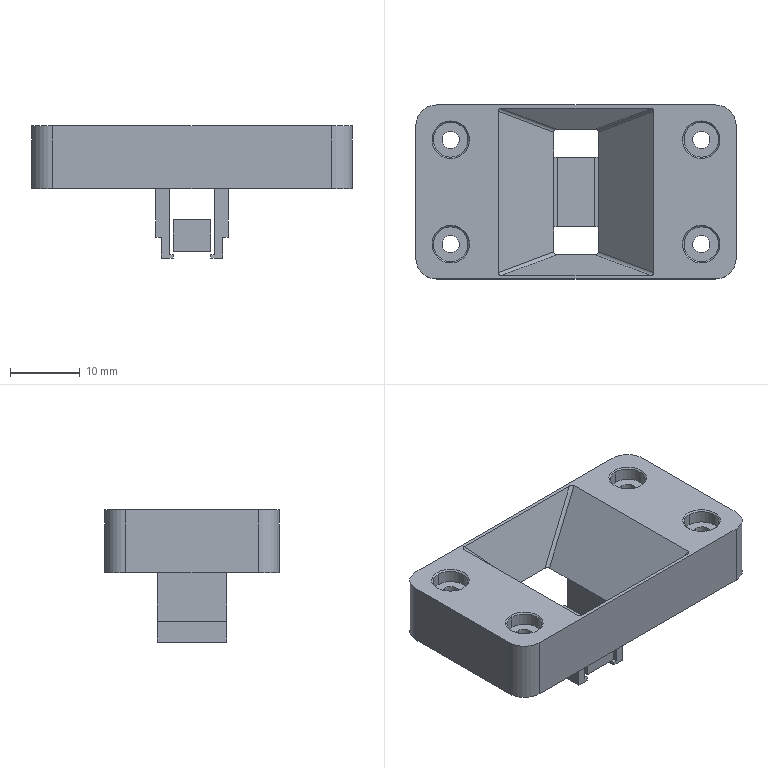NC program | NX | posted with a generic post | part box 46 x 25 x 19 mm
Lines 1575 to 3677 of 3737, first 1767 of 2099 lines:
(FIXED_CONTOUR_COPY , TOOL : D2R0.2)
N3094 T05 M6
N3096 G54
N3098 G17 G0 G90 X-10.255 Y11.119 S9500 M3
N3100 G43 Z30. H5
N3102 Z3.2
N3104 G94 G1 Z1.672 F500.
N3106 X-10.383 Y10.99 Z0.082
N3108 X-10.316 Y11.058 Z0.006 F2500.
N3110 X-10.3 Y11.073 Z0.052
N3112 X-10.229
N3114 X-10.264 Y11.039 Z-0.052
N3116 X-10.383 Y10.919 Z0.082
N3118 Y10.848
N3120 X-10.212 Y11.019 Z-0.11
N3122 X-10.158 Y11.073 Z0.052
N3124 X-10.087
N3126 X-10.161 Y11. Z-0.168
N3128 X-10.383 Y10.777 Z0.082
N3130 Y10.706
N3132 X-10.109 Y10.98 Z-0.226
N3134 X-10.016 Y11.073 Z0.053
N3136 X-9.945 Y11.074
N3138 X-10.058 Y10.961 Z-0.284
N3140 X-10.383 Y10.635 Z0.082
N3142 Y10.564
N3144 X-10.006 Y10.942 Z-0.342
N3146 X-9.874 Y11.074 Z0.053
N3148 X-9.803
N3150 X-9.954 Y10.922 Z-0.4
N3152 X-10.383 Y10.494 Z0.082
N3154 Y10.423
N3156 X-9.903 Y10.903 Z-0.458
N3158 X-9.732 Y11.074 Z0.053
N3160 X-9.662
N3162 X-9.851 Y10.884 Z-0.516
N3164 X-10.383 Y10.352 Z0.082
N3166 Y10.281
N3168 X-9.8 Y10.864 Z-0.574
N3170 X-9.591 Y11.074 Z0.053
N3172 X-9.52
N3174 X-9.748 Y10.845 Z-0.632
N3176 X-10.383 Y10.21 Z0.082
N3178 Y10.139
N3180 X-9.697 Y10.826 Z-0.69
N3182 X-9.449 Y11.074 Z0.053
N3184 X-9.378
N3186 X-9.645 Y10.806 Z-0.748
N3188 X-10.383 Y10.068 Z0.082
N3190 Y9.997
N3192 X-9.593 Y10.787 Z-0.806
N3194 X-9.307 Y11.074 Z0.053
N3196 X-9.236
N3198 X-9.542 Y10.768 Z-0.864
N3200 X-10.383 Y9.926 Z0.082
N3202 Y9.855
N3204 X-9.49 Y10.748 Z-0.922
N3206 X-9.165 Y11.074 Z0.053
N3208 X-9.094
N3210 X-9.439 Y10.729 Z-0.98
N3212 X-10.383 Y9.784 Z0.082
N3214 Y9.714
N3216 X-9.387 Y10.71 Z-1.038
N3218 X-9.023 Y11.074 Z0.053
N3220 X-8.952
N3222 X-9.336 Y10.69 Z-1.096
N3224 X-10.383 Y9.643 Z0.082
N3226 Y9.572
N3228 X-9.284 Y10.671 Z-1.154
N3230 X-8.881 Y11.074 Z0.053
N3232 X-8.811
N3234 X-9.232 Y10.652 Z-1.212
N3236 X-10.383 Y9.501 Z0.082
N3238 Y9.43
N3240 X-9.181 Y10.632 Z-1.27
N3242 X-8.74 Y11.074 Z0.053
N3244 X-8.669
N3246 X-9.129 Y10.613 Z-1.328
N3248 X-10.383 Y9.359 Z0.082
N3250 Y9.288
N3252 X-9.078 Y10.594 Z-1.387
N3254 X-8.598 Y11.074 Z0.053
N3256 X-8.527
N3258 X-9.026 Y10.574 Z-1.445
N3260 X-10.383 Y9.217 Z0.082
N3262 Y9.146
N3264 X-8.975 Y10.555 Z-1.503
N3266 X-8.456 Y11.074 Z0.053
N3268 X-8.385
N3270 X-8.923 Y10.536 Z-1.561
N3272 X-10.383 Y9.075 Z0.082
N3274 Y9.004
N3276 X-8.871 Y10.516 Z-1.619
N3278 X-8.314 Y11.074 Z0.053
N3280 X-8.243
N3282 X-8.82 Y10.497 Z-1.677
N3284 X-10.383 Y8.933 Z0.082
N3286 Y8.863
N3288 X-8.768 Y10.478 Z-1.735
N3290 X-8.172 Y11.074 Z0.053
N3292 X-8.101
N3294 X-8.717 Y10.458 Z-1.793
N3296 X-10.383 Y8.792 Z0.082
N3298 Y8.721
N3300 X-8.665 Y10.439 Z-1.851
N3302 X-8.031 Y11.074 Z0.053
N3304 X-7.96
N3306 X-8.614 Y10.42 Z-1.909
N3308 X-10.383 Y8.65 Z0.082
N3310 Y8.579
N3312 X-8.562 Y10.4 Z-1.967
N3314 X-7.889 Y11.074 Z0.053
N3316 X-7.818
N3318 X-8.51 Y10.381 Z-2.025
N3320 X-10.383 Y8.508 Z0.082
N3322 Y8.437
N3324 X-8.459 Y10.362 Z-2.083
N3326 X-7.747 Y11.074 Z0.053
N3328 X-7.676
N3330 X-8.407 Y10.342 Z-2.141
N3332 X-10.383 Y8.366 Z0.082
N3334 Y8.295
N3336 X-8.356 Y10.323 Z-2.199
N3338 X-7.605 Y11.074 Z0.053
N3340 X-7.534
N3342 X-8.304 Y10.304 Z-2.257
N3344 X-10.383 Y8.224 Z0.082
N3346 Y8.153
N3348 X-8.253 Y10.284 Z-2.315
N3350 X-7.463 Y11.074 Z0.053
N3352 X-7.392
N3354 X-8.201 Y10.265 Z-2.373
N3356 X-10.383 Y8.083 Z0.082
N3358 Y8.012
N3360 X-8.149 Y10.246 Z-2.431
N3362 X-7.321 Y11.074 Z0.053
N3364 X-7.251
N3366 X-8.098 Y10.226 Z-2.489
N3368 X-10.383 Y7.941 Z0.082
N3370 Y7.87
N3372 X-8.046 Y10.207 Z-2.547
N3374 X-7.18 Y11.074 Z0.053
N3376 X-7.109
N3378 X-7.995 Y10.188 Z-2.605
N3380 X-10.383 Y7.799 Z0.082
N3382 Y7.728
N3384 X-7.943 Y10.168 Z-2.663
N3386 X-7.038 Y11.074 Z0.053
N3388 X-6.967
N3390 X-7.892 Y10.149 Z-2.721
N3392 X-10.383 Y7.657 Z0.082
N3394 Y7.586
N3396 X-7.84 Y10.13 Z-2.779
N3398 X-6.896 Y11.074 Z0.053
N3400 X-6.825
N3402 X-7.788 Y10.11 Z-2.837
N3404 X-10.383 Y7.515 Z0.082
N3406 Y7.444
N3408 X-7.737 Y10.091 Z-2.895
N3410 X-6.754 Y11.074 Z0.053
N3412 X-6.683
N3414 X-7.685 Y10.072 Z-2.953
N3416 X-10.383 Y7.373 Z0.082
N3418 Y7.302
N3420 X-7.634 Y10.052 Z-3.011
N3422 X-6.612 Y11.074 Z0.053
N3424 X-6.541
N3426 X-7.582 Y10.033 Z-3.069
N3428 X-10.383 Y7.232 Z0.082
N3430 Y7.161
N3432 X-7.531 Y10.013 Z-3.127
N3434 X-6.47 Y11.074 Z0.053
N3436 X-6.4
N3438 X-7.479 Y9.994 Z-3.185
N3440 X-10.383 Y7.09 Z0.082
N3442 Y7.019
N3444 X-7.427 Y9.975 Z-3.243
N3446 X-6.329 Y11.074 Z0.053
N3448 X-6.258
N3450 X-7.376 Y9.955 Z-3.301
N3452 X-10.383 Y6.948 Z0.082
N3454 Y6.877
N3456 X-7.324 Y9.936 Z-3.359
N3458 X-6.187 Y11.074 Z0.053
N3460 X-6.116
N3462 X-7.273 Y9.917 Z-3.417
N3464 X-10.383 Y6.806 Z0.082
N3466 Y6.735
N3468 X-7.221 Y9.897 Z-3.475
N3470 X-6.045 Y11.074 Z0.053
N3472 X-5.974
N3474 X-7.17 Y9.878 Z-3.533
N3476 X-10.383 Y6.664 Z0.082
N3478 Y6.593
N3480 X-7.118 Y9.859 Z-3.591
N3482 X-5.903 Y11.074 Z0.053
N3484 X-5.832
N3486 X-7.066 Y9.839 Z-3.649
N3488 X-10.383 Y6.522 Z0.082
N3490 Y6.452
N3492 X-7.015 Y9.82 Z-3.707
N3494 X-5.761 Y11.074 Z0.053
N3496 X-5.69
N3498 X-6.963 Y9.801 Z-3.765
N3500 X-10.383 Y6.381 Z0.082
N3502 Y6.31
N3504 X-6.912 Y9.781 Z-3.823
N3506 X-5.62 Y11.074 Z0.053
N3508 X-5.549
N3510 X-6.86 Y9.762 Z-3.881
N3512 X-10.383 Y6.239 Z0.082
N3514 Y6.168
N3516 X-6.809 Y9.743 Z-3.939
N3518 X-5.478 Y11.074 Z0.053
N3520 X-5.407
N3522 X-6.757 Y9.723 Z-3.997
N3524 X-10.383 Y6.097 Z0.082
N3526 Y6.026
N3528 X-6.705 Y9.704 Z-4.055
N3530 X-5.336 Y11.074 Z0.053
N3532 X-5.265
N3534 X-6.654 Y9.685 Z-4.113
N3536 X-10.383 Y5.955 Z0.082
N3538 Y5.884
N3540 X-6.602 Y9.665 Z-4.171
N3542 X-5.194 Y11.074 Z0.053
N3544 X-5.123
N3546 X-6.551 Y9.646 Z-4.229
N3548 X-10.383 Y5.813 Z0.082
N3550 Y5.742
N3552 X-6.499 Y9.627 Z-4.287
N3554 X-5.052 Y11.074 Z0.053
N3556 X-4.981
N3558 X-6.448 Y9.607 Z-4.345
N3560 X-10.383 Y5.671 Z0.082
N3562 Y5.601
N3564 X-6.396 Y9.588 Z-4.404
N3566 X-4.91 Y11.074 Z0.053
N3568 X-4.839
N3570 X-6.344 Y9.569 Z-4.462
N3572 X-10.383 Y5.53 Z0.082
N3574 Y5.459
N3576 X-6.293 Y9.549 Z-4.52
N3578 X-4.769 Y11.074 Z0.053
N3580 X-4.698
N3582 X-6.241 Y9.53 Z-4.578
N3584 X-10.383 Y5.388 Z0.082
N3586 Y5.317
N3588 X-6.19 Y9.511 Z-4.636
N3590 X-4.627 Y11.074 Z0.053
N3592 X-4.556
N3594 X-6.138 Y9.491 Z-4.694
N3596 X-10.383 Y5.246 Z0.082
N3598 Y5.175
N3600 X-6.087 Y9.472 Z-4.752
N3602 X-4.485 Y11.074 Z0.053
N3604 X-4.414
N3606 X-6.035 Y9.453 Z-4.81
N3608 X-10.383 Y5.104 Z0.082
N3610 Y5.033
N3612 X-5.983 Y9.433 Z-4.868
N3614 X-4.343 Y11.074 Z0.053
N3616 X-4.272
N3618 X-5.932 Y9.414 Z-4.926
N3620 X-10.383 Y4.962 Z0.082
N3622 Y4.891
N3624 X-5.88 Y9.395 Z-4.984
N3626 X-4.201 Y11.074 Z0.053
N3628 X-4.13
N3630 X-5.829 Y9.375 Z-5.042
N3632 X-10.383 Y4.821 Z0.082
N3634 Y4.75
N3636 X-5.777 Y9.356 Z-5.1
N3638 X-4.059 Y11.074 Z0.053
N3640 X-3.989
N3642 X-5.726 Y9.337 Z-5.158
N3644 X-10.383 Y4.679 Z0.082
N3646 Y4.608
N3648 X-5.674 Y9.317 Z-5.216
N3650 X-3.918 Y11.074 Z0.053
N3652 X-3.847
N3654 X-5.622 Y9.298 Z-5.274
N3656 X-10.383 Y4.537 Z0.082
N3658 Y4.466
N3660 X-5.571 Y9.279 Z-5.332
N3662 X-3.776 Y11.074 Z0.053
N3664 X-3.705
N3666 X-5.519 Y9.259 Z-5.39
N3668 X-10.383 Y4.395 Z0.082
N3670 Y4.324
N3672 X-5.468 Y9.24 Z-5.448
N3674 X-3.634 Y11.074 Z0.053
N3676 X-3.563
N3678 X-5.416 Y9.221 Z-5.506
N3680 X-10.383 Y4.253 Z0.082
N3682 Y4.182
N3684 X-5.365 Y9.201 Z-5.564
N3686 X-3.492 Y11.074 Z0.053
N3688 X-3.421
N3690 X-5.313 Y9.182 Z-5.622
N3692 X-10.383 Y4.111 Z0.082
N3694 Y4.04
N3696 X-5.261 Y9.163 Z-5.68
N3698 X-3.35 Y11.074 Z0.053
N3700 X-3.279
N3702 X-5.21 Y9.143 Z-5.738
N3704 X-10.383 Y3.97 Z0.082
N3706 Y3.899
N3708 X-5.158 Y9.124 Z-5.796
N3710 X-3.209 Y11.074 Z0.053
N3712 X-3.138
N3714 X-5.107 Y9.105 Z-5.854
N3716 X-10.383 Y3.828 Z0.082
N3718 Y3.757
N3720 X-5.055 Y9.085 Z-5.912
N3722 X-3.067 Y11.074 Z0.053
N3724 X-2.996
N3726 X-5.003 Y9.066 Z-5.97
N3728 X-10.383 Y3.686 Z0.082
N3730 Y3.615
N3732 X-4.952 Y9.046 Z-6.028
N3734 X-2.925 Y11.074 Z0.053
N3736 X-2.854
N3738 X-4.9 Y9.027 Z-6.086
N3740 X-10.383 Y3.544 Z0.082
N3742 Y3.473
N3744 X-4.849 Y9.008 Z-6.144
N3746 X-2.783 Y11.074 Z0.053
N3748 X-2.712
N3750 X-4.797 Y8.988 Z-6.202
N3752 X-10.383 Y3.402 Z0.082
N3754 Y3.331
N3756 X-4.746 Y8.969 Z-6.26
N3758 X-2.641 Y11.074 Z0.053
N3760 X-2.57
N3762 X-4.694 Y8.95 Z-6.318
N3764 X-10.383 Y3.26 Z0.082
N3766 Y3.19
N3768 X-4.642 Y8.93 Z-6.376
N3770 X-2.499 Y11.074 Z0.053
N3772 X-2.428
N3774 X-4.591 Y8.911 Z-6.434
N3776 X-10.383 Y3.119 Z0.082
N3778 Y3.048
N3780 X-4.539 Y8.892 Z-6.492
N3782 X-2.358 Y11.074 Z0.053
N3784 X-2.287
N3786 X-4.488 Y8.872 Z-6.55
N3788 X-10.383 Y2.977 Z0.082
N3790 Y2.906
N3792 X-4.436 Y8.853 Z-6.608
N3794 X-2.216 Y11.074 Z0.053
N3796 X-2.145
N3798 X-4.385 Y8.834 Z-6.666
N3800 X-10.383 Y2.835 Z0.082
N3802 Y2.764
N3804 X-4.333 Y8.814 Z-6.724
N3806 X-2.074 Y11.074 Z0.053
N3808 X-2.003
N3810 X-4.281 Y8.795 Z-6.782
N3812 X-10.383 Y2.693 Z0.082
N3814 Y2.622
N3816 X-4.23 Y8.776 Z-6.84
N3818 X-1.932 Y11.074 Z0.053
N3820 X-1.861
N3822 X-4.178 Y8.756 Z-6.898
N3824 X-10.383 Y2.551 Z0.082
N3826 Y2.48
N3828 X-4.127 Y8.737 Z-6.956
N3830 X-1.79 Y11.074 Z0.053
N3832 X-1.719
N3834 X-4.075 Y8.718 Z-7.014
N3836 X-10.383 Y2.409 Z0.082
N3838 Y2.339
N3840 X-4.024 Y8.698 Z-7.072
N3842 X-1.648 Y11.074 Z0.053
N3844 X-1.578
N3846 X-3.972 Y8.679 Z-7.13
N3848 X-10.383 Y2.268 Z0.082
N3850 Y2.197
N3852 X-3.92 Y8.66 Z-7.188
N3854 X-1.507 Y11.074 Z0.053
N3856 X-1.436
N3858 X-3.869 Y8.64 Z-7.246
N3860 X-10.383 Y2.126 Z0.082
N3862 Y2.055
N3864 X-3.817 Y8.621 Z-7.304
N3866 X-1.365 Y11.074 Z0.053
N3868 X-1.294
N3870 X-3.766 Y8.602 Z-7.362
N3872 X-10.383 Y1.984 Z0.082
N3874 Y1.913
N3876 X-3.714 Y8.582 Z-7.421
N3878 X-1.223 Y11.074 Z0.053
N3880 X-1.152
N3882 X-3.663 Y8.563 Z-7.479
N3884 X-10.383 Y1.842 Z0.082
N3886 Y1.771
N3888 X-3.611 Y8.544 Z-7.537
N3890 X-1.081 Y11.074 Z0.053
N3892 X-1.01
N3894 X-3.559 Y8.524 Z-7.595
N3896 X-10.383 Y1.7 Z0.082
N3898 Y1.629
N3900 X-3.508 Y8.505 Z-7.653
N3902 X-0.939 Y11.074 Z0.053
N3904 X-0.868
N3906 X-3.456 Y8.486 Z-7.711
N3908 X-10.383 Y1.559 Z0.082
N3910 Y1.488
N3912 X-3.405 Y8.466 Z-7.769
N3914 X-0.797 Y11.074 Z0.053
N3916 X-0.727
N3918 X-3.353 Y8.447 Z-7.827
N3920 X-10.383 Y1.417 Z0.082
N3922 Y1.346
N3924 X-3.302 Y8.428 Z-7.885
N3926 X-0.656 Y11.074 Z0.053
N3928 X-0.585
N3930 X-3.25 Y8.408 Z-7.943
N3932 X-10.383 Y1.275 Z0.082
N3934 Y1.204
N3936 X-3.198 Y8.389 Z-8.001
N3938 X-0.514 Y11.074 Z0.053
N3940 X-0.443
N3942 X-3.147 Y8.37 Z-8.059
N3944 X-10.383 Y1.133 Z0.082
N3946 Y1.062
N3948 X-3.095 Y8.35 Z-8.117
N3950 X-0.372 Y11.074 Z0.053
N3952 X-0.301
N3954 X-3.044 Y8.331 Z-8.175
N3956 X-10.383 Y0.991 Z0.082
N3958 Y0.92
N3960 X-2.992 Y8.312 Z-8.233
N3962 X-0.23 Y11.074 Z0.053
N3964 X-0.159
N3966 X-2.941 Y8.292 Z-8.291
N3968 X-10.383 Y0.849 Z0.082
N3970 Y0.779
N3972 X-2.889 Y8.273 Z-8.349
N3974 X-0.088 Y11.074 Z0.053
N3976 X-0.017
N3978 X-2.837 Y8.254 Z-8.407
N3980 X-10.383 Y0.708 Z0.082
N3982 Y0.637
N3984 X-2.786 Y8.234 Z-8.465
N3986 X0.053 Y11.074 Z0.053
N3988 X0.124
N3990 X-2.734 Y8.215 Z-8.523
N3992 X-10.383 Y0.566 Z0.082
N3994 Y0.495
N3996 X-2.683 Y8.196 Z-8.581
N3998 X0.195 Y11.074 Z0.053
N4000 X0.266
N4002 X-2.631 Y8.176 Z-8.639
N4004 X-10.383 Y0.424 Z0.082
N4006 Y0.353
N4008 X-2.58 Y8.157 Z-8.697
N4010 X0.337 Y11.074 Z0.053
N4012 X0.408
N4014 X-2.528 Y8.138 Z-8.755
N4016 X-10.383 Y0.282 Z0.082
N4018 Y0.211
N4020 X-2.476 Y8.118 Z-8.813
N4022 X0.479 Y11.074 Z0.053
N4024 X0.55
N4026 X-2.425 Y8.099 Z-8.871
N4028 X-10.383 Y0.14 Z0.082
N4030 Y0.069
N4032 X-2.373 Y8.08 Z-8.929
N4034 X0.621 Y11.074 Z0.053
N4036 X0.692
N4038 X-2.322 Y8.06 Z-8.987
N4040 X-10.383 Y-0.002 Z0.082
N4042 Y-0.072
N4044 X-2.27 Y8.041 Z-9.045
N4046 X0.763 Y11.074 Z0.053
N4048 X0.834
N4050 X-2.219 Y8.021 Z-9.103
N4052 X-10.383 Y-0.143 Z0.082
N4054 Y-0.214
N4056 X-2.167 Y8.002 Z-9.161
N4058 X0.904 Y11.074 Z0.053
N4060 X0.988
N4062 X-2.106 Y7.979 Z-9.231
N4064 X-2.1 Y7.976 Z-9.239
N4066 X-2.085 Y7.967 Z-9.266
N4068 X-2.084 Y7.966 Z-9.269
N4070 X-2.083 Z-9.271
N4072 X-2.077 Y7.96 Z-9.288
N4074 X-2.072 Y7.956 Z-9.3
N4076 X-2.068 Y7.947 Z-9.326
N4078 X-2.054
N4080 X1.072 Y11.074 Z0.053
N4082 X1.156
N4084 X-1.97 Y7.947 Z-9.326
N4086 X-1.887
N4088 X1.24 Y11.074 Z0.053
N4090 X1.324
N4092 X-1.803 Y7.947 Z-9.326
N4094 X-1.719
N4096 X1.408 Y11.074 Z0.053
N4098 X1.492
N4100 X-1.635 Y7.947 Z-9.326
N4102 X-1.551
N4104 X1.576 Y11.074 Z0.053
N4106 X1.66
N4108 X-1.467 Y7.947 Z-9.326
N4110 X-1.383
N4112 X1.743 Y11.074 Z0.053
N4114 X1.827
N4116 X-1.299 Y7.947 Z-9.326
N4118 X-1.215
N4120 X1.911 Y11.074 Z0.053
N4122 X1.995
N4124 X-1.132 Y7.947 Z-9.326
N4126 X-1.048
N4128 X2.079 Y11.074 Z0.053
N4130 X2.163
N4132 X-0.964 Y7.947 Z-9.326
N4134 X-0.88
N4136 X2.247 Y11.074 Z0.053
N4138 X2.331
N4140 X-0.796 Y7.947 Z-9.326
N4142 X-0.712
N4144 X2.415 Y11.074 Z0.053
N4146 X2.499
N4148 X-0.628 Y7.947 Z-9.326
N4150 X-0.544
N4152 X2.582 Y11.074 Z0.053
N4154 X2.666
N4156 X-0.46 Y7.947 Z-9.326
N4158 X-0.376
N4160 X2.75 Y11.074 Z0.053
N4162 X2.834
N4164 X-0.293 Y7.947 Z-9.326
N4166 X-0.209
N4168 X2.918 Y11.074 Z0.053
N4170 X3.002
N4172 X-0.125 Y7.947 Z-9.326
N4174 X-0.041
N4176 X3.086 Y11.074 Z0.053
N4178 X3.17
N4180 X0.043 Y7.947 Z-9.326
N4182 X0.127
N4184 X3.254 Y11.074 Z0.053
N4186 X3.337
N4188 X0.211 Y7.947 Z-9.326
N4190 X0.295
N4192 X3.421 Y11.074 Z0.053
N4194 X3.505
N4196 X0.379 Y7.947 Z-9.326
N4198 X0.463
N4200 X3.589 Y11.074 Z0.053
N4202 X3.673
N4204 X0.546 Y7.947 Z-9.326
N4206 X0.63
N4208 X3.757 Y11.074 Z0.053
N4210 X3.841
N4212 X0.714 Y7.947 Z-9.326
N4214 X0.798
N4216 X3.925 Y11.074 Z0.053
N4218 X4.009
N4220 X0.882 Y7.947 Z-9.326
N4222 X0.966
N4224 X4.093 Y11.074 Z0.053
N4226 X4.176
N4228 X1.05 Y7.947 Z-9.326
N4230 X1.134
N4232 X4.26 Y11.074 Z0.053
N4234 X4.344
N4236 X1.218 Y7.947 Z-9.326
N4238 X1.302
N4240 X4.428 Y11.074 Z0.053
N4242 X4.512
N4244 X1.385 Y7.947 Z-9.326
N4246 X1.469
N4248 X4.596 Y11.074 Z0.053
N4250 X4.68
N4252 X1.553 Y7.947 Z-9.326
N4254 X1.637
N4256 X4.764 Y11.074 Z0.053
N4258 X4.848
N4260 X1.721 Y7.947 Z-9.326
N4262 X1.805
N4264 X4.932 Y11.074 Z0.053
N4266 X5.015
N4268 X1.889 Y7.947 Z-9.326
N4270 X1.973
N4272 X5.099 Y11.074 Z0.053
N4274 X5.183
N4276 X2.057 Y7.947 Z-9.326
N4278 X2.068
N4280 X2.072 Y7.956 Z-9.3
N4282 X2.077 Y7.96 Z-9.288
N4284 X2.078 Y7.961 Z-9.285
N4286 X2.08 Y7.962 Z-9.281
N4288 X2.083 Y7.966 Z-9.271
N4290 X2.086 Y7.967 Z-9.266
N4292 X2.089 Y7.969 Z-9.259
N4294 X2.1 Y7.976 Z-9.239
N4296 X2.118 Y7.984 Z-9.215
N4298 Z-9.217
N4300 Y7.924
N4302 X2.213 Y8.019 Z-9.109
N4304 X5.267 Y11.074 Z0.053
N4306 X5.351
N4308 X2.347 Y8.07 Z-8.958
N4310 X2.118 Y7.84 Z-9.217
N4312 Y7.756
N4314 X2.482 Y8.12 Z-8.807
N4316 X5.435 Y11.074 Z0.053
N4318 X5.519
N4320 X2.616 Y8.17 Z-8.656
N4322 X2.118 Y7.672 Z-9.217
N4324 Y7.588
N4326 X2.75 Y8.221 Z-8.505
N4328 X5.603 Y11.074 Z0.053
N4330 X5.687
N4332 X2.884 Y8.271 Z-8.354
N4334 X2.118 Y7.504 Z-9.217
N4336 Y7.421
N4338 X3.018 Y8.321 Z-8.203
N4340 X5.771 Y11.074 Z0.053
N4342 X5.854
N4344 X3.153 Y8.372 Z-8.052
N4346 X2.118 Y7.337 Z-9.217
N4348 Y7.253
N4350 X3.287 Y8.422 Z-7.901
N4352 X5.938 Y11.074 Z0.053
N4354 X6.022
N4356 X3.421 Y8.472 Z-7.75
N4358 X2.118 Y7.169 Z-9.217
N4360 Y7.096
N4362 Y5.966 Z-8.085
N4364 Z-4.635
N4366 G0 Z-1.835
N4368 X1.924 Y7.033
N4370 Z-2.235
N4372 G1 Z-9.217 F500.
N4374 G3 X2.118 Y7.085 R0.2
N4376 G1 X3.555 Y8.523 Z-7.599 F2500.
N4378 X6.106 Y11.074 Z0.053
N4380 X6.19
N4382 X3.69 Y8.573 Z-7.448
N4384 X2.118 Y7.001 Z-9.217
N4386 Y6.917
N4388 X3.824 Y8.624 Z-7.297
N4390 X6.274 Y11.074 Z0.053
N4392 X6.358
N4394 X3.958 Y8.674 Z-7.146
N4396 X2.118 Y6.833 Z-9.217
N4398 Y6.749
N4400 X4.092 Y8.724 Z-6.995
N4402 X6.442 Y11.074 Z0.053
N4404 X6.526
N4406 X4.227 Y8.775 Z-6.844
N4408 X2.118 Y6.665 Z-9.217
N4410 Y6.582
N4412 X4.361 Y8.825 Z-6.693
N4414 X6.61 Y11.074 Z0.053
N4416 X6.694
N4418 X4.495 Y8.875 Z-6.542
N4420 X2.118 Y6.498 Z-9.217
N4422 Y6.414
N4424 X4.629 Y8.926 Z-6.391
N4426 X6.777 Y11.074 Z0.053
N4428 X6.861
N4430 X4.764 Y8.976 Z-6.24
N4432 X2.118 Y6.33 Z-9.217
N4434 Y6.246
N4436 X4.898 Y9.026 Z-6.089
N4438 X6.945 Y11.074 Z0.053
N4440 X7.029
N4442 X5.032 Y9.077 Z-5.938
N4444 X2.118 Y6.162 Z-9.217
N4446 Y6.078
N4448 X5.166 Y9.127 Z-5.787
N4450 X7.113 Y11.074 Z0.053
N4452 X7.197
N4454 X5.301 Y9.177 Z-5.636
N4456 X2.118 Y5.994 Z-9.217
N4458 Y5.91
N4460 X5.435 Y9.228 Z-5.485
N4462 X7.281 Y11.074 Z0.053
N4464 X7.365
N4466 X5.569 Y9.278 Z-5.334
N4468 X2.118 Y5.826 Z-9.217
N4470 Y5.742
N4472 X5.703 Y9.328 Z-5.183
N4474 X7.449 Y11.074 Z0.053
N4476 X7.533
N4478 X5.838 Y9.379 Z-5.032
N4480 X2.118 Y5.659 Z-9.217
N4482 Y5.575
N4484 X5.972 Y9.429 Z-4.881
N4486 X7.616 Y11.074 Z0.053
N4488 X7.7
N4490 X6.106 Y9.479 Z-4.73
N4492 X2.118 Y5.491 Z-9.217
N4494 Y5.407
N4496 X6.24 Y9.53 Z-4.579
N4498 X7.784 Y11.074 Z0.053
N4500 X7.868
N4502 X6.375 Y9.58 Z-4.428
N4504 X2.118 Y5.323 Z-9.217
N4506 Y5.239
N4508 X6.509 Y9.63 Z-4.276
N4510 X7.952 Y11.074 Z0.053
N4512 X8.036
N4514 X6.643 Y9.681 Z-4.126
N4516 X2.118 Y5.155 Z-9.217
N4518 Y5.071
N4520 X6.777 Y9.731 Z-3.974
N4522 X8.12 Y11.074 Z0.053
N4524 X8.204
N4526 X6.912 Y9.781 Z-3.823
N4528 X2.118 Y4.987 Z-9.217
N4530 Y4.903
N4532 X7.046 Y9.832 Z-3.672
N4534 X8.288 Y11.074 Z0.053
N4536 X8.372
N4538 X7.18 Y9.882 Z-3.521
N4540 X2.118 Y4.82 Z-9.217
N4542 Y4.736
N4544 X7.314 Y9.932 Z-3.37
N4546 X8.455 Y11.074 Z0.053
N4548 X8.539
N4550 X7.449 Y9.983 Z-3.219
N4552 X2.118 Y4.652 Z-9.217
N4554 Y4.568
N4556 X7.583 Y10.033 Z-3.068
N4558 X8.623 Y11.074 Z0.053
N4560 X8.707
N4562 X7.717 Y10.083 Z-2.917
N4564 X2.118 Y4.484 Z-9.217
N4566 Y4.4
N4568 X7.851 Y10.134 Z-2.766
N4570 X8.791 Y11.074 Z0.053
N4572 X8.875
N4574 X7.986 Y10.184 Z-2.615
N4576 X2.118 Y4.316 Z-9.217
N4578 Y4.232
N4580 X8.12 Y10.234 Z-2.464
N4582 X8.959 Y11.074 Z0.053
N4584 X9.043
N4586 X8.254 Y10.285 Z-2.313
N4588 X2.118 Y4.148 Z-9.217
N4590 Y4.064
N4592 X8.388 Y10.335 Z-2.162
N4594 X9.127 Y11.074 Z0.053
N4596 X9.211
N4598 X8.523 Y10.385 Z-2.011
N4600 X2.118 Y3.981 Z-9.217
N4602 Y3.897
N4604 X8.657 Y10.436 Z-1.86
N4606 X9.295 Y11.074 Z0.053
N4608 X9.378
N4610 X8.791 Y10.486 Z-1.709
N4612 X2.118 Y3.813 Z-9.217
N4614 Y3.729
N4616 X8.925 Y10.537 Z-1.558
N4618 X9.462 Y11.074 Z0.053
N4620 X9.546
N4622 X9.06 Y10.587 Z-1.407
N4624 X2.118 Y3.645 Z-9.217
N4626 Y3.561
N4628 X9.194 Y10.637 Z-1.256
N4630 X9.63 Y11.074 Z0.053
N4632 X9.714
N4634 X9.328 Y10.688 Z-1.105
N4636 X2.118 Y3.477 Z-9.217
N4638 Y3.393
N4640 X9.462 Y10.738 Z-0.954
N4642 X9.798 Y11.074 Z0.053
N4644 X9.882
N4646 X9.597 Y10.788 Z-0.803
N4648 X2.118 Y3.309 Z-9.217
N4650 Y3.225
N4652 X9.731 Y10.839 Z-0.652
N4654 X9.966 Y11.073 Z0.053
N4656 X10.05
N4658 X9.865 Y10.889 Z-0.501
N4660 X2.118 Y3.141 Z-9.217
N4662 Y3.058
N4664 X9.999 Y10.939 Z-0.35
N4666 X10.133 Y11.073 Z0.052
N4668 X10.217
N4670 X10.134 Y10.99 Z-0.199
N4672 X2.118 Y2.974 Z-9.217
N4674 Y2.89
N4676 X10.268 Y11.04 Z-0.048
N4678 X10.301 Y11.073 Z0.052
N4680 X10.356
N4682 X10.367 Y11.078 Z0.063
N4684 X10.383 Y11.086 Z0.082
N4686 Y11.06
N4688 X9.997 Y10.673 Z-0.353
N4690 X2.118 Y2.794 Z-9.217
N4692 Y2.699
N4694 X10.383 Y10.964 Z0.082
N4696 Y10.869
N4698 X2.118 Y2.603 Z-9.217
N4700 Y2.508
N4702 X10.383 Y10.773 Z0.082
N4704 Y10.678
N4706 X2.118 Y2.412 Z-9.217
N4708 Y2.317
N4710 X10.383 Y10.583 Z0.082
N4712 Y10.487
N4714 X2.118 Y2.221 Z-9.217
N4716 Y2.126
N4718 X10.383 Y10.392 Z0.082
N4720 Y10.296
N4722 X2.118 Y2.03 Z-9.217
N4724 Y1.935
N4726 X10.383 Y10.201 Z0.082
N4728 Y10.105
N4730 X2.118 Y1.839 Z-9.217
N4732 Y1.744
N4734 X10.383 Y10.01 Z0.082
N4736 Y9.914
N4738 X2.118 Y1.648 Z-9.217
N4740 Y1.553
N4742 X10.383 Y9.819 Z0.082
N4744 Y9.723
N4746 X2.118 Y1.457 Z-9.217
N4748 Y1.362
N4750 X10.383 Y9.628 Z0.082
N4752 Y9.544
N4754 X2.118 Y1.278 Z-9.217
N4756 Y1.194
N4758 X10.383 Y9.46 Z0.082
N4760 Y9.376
N4762 X2.118 Y1.11 Z-9.217
N4764 Y1.026
N4766 X10.383 Y9.292 Z0.082
N4768 Y9.208
N4770 X2.118 Y0.942 Z-9.217
N4772 Y0.858
N4774 X10.383 Y9.124 Z0.082
N4776 Y9.04
N4778 X2.118 Y0.774 Z-9.217
N4780 Y0.69
N4782 X10.383 Y8.956 Z0.082
N4784 Y8.872
N4786 X2.118 Y0.607 Z-9.217
N4788 Y0.523
N4790 X10.383 Y8.788 Z0.082
N4792 Y8.705
N4794 X2.118 Y0.439 Z-9.217
N4796 Y0.355
N4798 X10.383 Y8.621 Z0.082
N4800 Y8.537
N4802 X2.118 Y0.271 Z-9.217
N4804 Y0.187
N4806 X10.383 Y8.453 Z0.082
N4808 Y8.369
N4810 X2.118 Y0.103 Z-9.217
N4812 Y0.019
N4814 X10.383 Y8.285 Z0.082
N4816 Y8.201
N4818 X2.118 Y-0.065 Z-9.217
N4820 Y-0.149
N4822 X10.383 Y8.117 Z0.082
N4824 Y8.033
N4826 X2.118 Y-0.232 Z-9.217
N4828 Y-0.316
N4830 X10.383 Y7.949 Z0.082
N4832 Y7.866
N4834 X2.118 Y-0.4 Z-9.217
N4836 Y-0.484
N4838 X10.383 Y7.782 Z0.082
N4840 Y7.698
N4842 X2.118 Y-0.568 Z-9.217
N4844 Y-0.652
N4846 X10.383 Y7.614 Z0.082
N4848 Y7.53
N4850 X2.118 Y-0.736 Z-9.217
N4852 Y-0.82
N4854 X10.383 Y7.446 Z0.082
N4856 Y7.362
N4858 X2.118 Y-0.904 Z-9.217
N4860 Y-0.988
N4862 X10.383 Y7.278 Z0.082
N4864 Y7.194
N4866 X2.118 Y-1.071 Z-9.217
N4868 Y-1.155
N4870 X10.383 Y7.11 Z0.082
N4872 Y7.027
N4874 X2.118 Y-1.239 Z-9.217
N4876 Y-1.323
N4878 X10.383 Y6.943 Z0.082
N4880 Y6.859
N4882 X2.118 Y-1.407 Z-9.217
N4884 Y-1.491
N4886 X10.383 Y6.775 Z0.082
N4888 Y6.691
N4890 X2.118 Y-1.575 Z-9.217
N4892 Y-1.659
N4894 X10.383 Y6.607 Z0.082
N4896 Y6.523
N4898 X2.118 Y-1.743 Z-9.217
N4900 Y-1.827
N4902 X10.383 Y6.439 Z0.082
N4904 Y6.355
N4906 X2.118 Y-1.91 Z-9.217
N4908 Y-1.994
N4910 X10.383 Y6.271 Z0.082
N4912 Y6.188
N4914 X2.118 Y-2.078 Z-9.217
N4916 Y-2.162
N4918 X10.383 Y6.104 Z0.082
N4920 Y6.02
N4922 X2.118 Y-2.246 Z-9.217
N4924 Y-2.33
N4926 X10.383 Y5.936 Z0.082
N4928 Y5.852
N4930 X2.118 Y-2.414 Z-9.217
N4932 Y-2.498
N4934 X10.383 Y5.768 Z0.082
N4936 Y5.684
N4938 X2.118 Y-2.582 Z-9.217
N4940 Y-2.666
N4942 X10.383 Y5.6 Z0.082
N4944 Y5.516
N4946 X2.118 Y-2.75 Z-9.217
N4948 Y-2.833
N4950 X10.383 Y5.432 Z0.082
N4952 Y5.349
N4954 X2.118 Y-2.917 Z-9.217
N4956 Y-3.001
N4958 X10.383 Y5.265 Z0.082
N4960 Y5.181
N4962 X2.118 Y-3.085 Z-9.217
N4964 Y-3.169
N4966 X10.383 Y5.097 Z0.082
N4968 Y5.013
N4970 X2.118 Y-3.253 Z-9.217
N4972 Y-3.337
N4974 X10.383 Y4.929 Z0.082
N4976 Y4.845
N4978 X2.118 Y-3.421 Z-9.217
N4980 Y-3.505
N4982 X10.383 Y4.761 Z0.082
N4984 Y4.677
N4986 X2.118 Y-3.589 Z-9.217
N4988 Y-3.672
N4990 X10.383 Y4.593 Z0.082
N4992 Y4.51
N4994 X2.118 Y-3.756 Z-9.217
N4996 Y-3.84
N4998 X10.383 Y4.426 Z0.082
N5000 Y4.343
N5002 X2.118 Y-3.923 Z-9.217
N5004 Y-4.005
N5006 X10.383 Y4.261 Z0.082
N5008 Y4.179
N5010 X2.118 Y-4.087 Z-9.217
N5012 Y-4.169
N5014 X10.383 Y4.096 Z0.082
N5016 Y4.014
N5018 X2.118 Y-4.252 Z-9.217
N5020 Y-4.334
N5022 X10.383 Y3.932 Z0.082
N5024 Y3.849
N5026 X2.118 Y-4.416 Z-9.217
N5028 Y-4.499
N5030 X10.383 Y3.767 Z0.082
N5032 Y3.685
N5034 X2.118 Y-4.581 Z-9.217
N5036 Y-4.663
N5038 X10.383 Y3.602 Z0.082
N5040 Y3.52
N5042 X2.118 Y-4.746 Z-9.217
N5044 Y-4.828
N5046 X10.383 Y3.438 Z0.082
N5048 Y3.356
N5050 X2.118 Y-4.91 Z-9.217
N5052 Y-4.993
N5054 X10.383 Y3.273 Z0.082
N5056 Y3.191
N5058 X2.118 Y-5.075 Z-9.217
N5060 Y-5.157
N5062 X10.383 Y3.109 Z0.082
N5064 Y3.026
N5066 X2.118 Y-5.24 Z-9.217
N5068 Y-5.322
N5070 X10.383 Y2.944 Z0.082
N5072 Y2.862
N5074 X2.118 Y-5.404 Z-9.217
N5076 Y-5.487
N5078 X10.383 Y2.779 Z0.082
N5080 Y2.697
N5082 X2.118 Y-5.569 Z-9.217
N5084 Y-5.651
N5086 X10.383 Y2.615 Z0.082
N5088 Y2.532
N5090 X2.118 Y-5.733 Z-9.217
N5092 Y-5.816
N5094 X10.383 Y2.45 Z0.082
N5096 Y2.368
N5098 X2.118 Y-5.898 Z-9.217
N5100 Y-5.98
N5102 X10.383 Y2.285 Z0.082
N5104 Y2.203
N5106 X2.118 Y-6.063 Z-9.217
N5108 Y-6.145
N5110 X10.383 Y2.121 Z0.082
N5112 Y2.038
N5114 X2.118 Y-6.227 Z-9.217
N5116 Y-6.31
N5118 X10.383 Y1.956 Z0.082
N5120 Y1.874
N5122 X2.118 Y-6.392 Z-9.217
N5124 Y-6.474
N5126 X10.383 Y1.791 Z0.082
N5128 Y1.709
N5130 X2.118 Y-6.557 Z-9.217
N5132 Y-6.639
N5134 X10.383 Y1.627 Z0.082
N5136 Y1.544
N5138 X2.118 Y-6.721 Z-9.217
N5140 Y-6.804
N5142 X10.383 Y1.462 Z0.082
N5144 Y1.38
N5146 X2.118 Y-6.886 Z-9.217
N5148 Y-6.969
N5150 X10.383 Y1.297 Z0.082
N5152 Y1.215
N5154 X2.118 Y-7.051 Z-9.217
N5156 Y-7.133
N5158 X10.383 Y1.133 Z0.082
N5160 Y1.05
N5162 X2.118 Y-7.216 Z-9.217
N5164 Y-7.298
N5166 X10.383 Y0.968 Z0.082
N5168 Y0.886
N5170 X2.118 Y-7.38 Z-9.217
N5172 Y-7.463
N5174 X10.383 Y0.803 Z0.082
N5176 Y0.721
N5178 X2.118 Y-7.545 Z-9.217
N5180 Y-7.627
N5182 X10.383 Y0.639 Z0.082
N5184 Y0.556
N5186 X2.118 Y-7.71 Z-9.217
N5188 Y-7.792
N5190 X10.383 Y0.474 Z0.082
N5192 Y0.391
N5194 X2.118 Y-7.874 Z-9.217
N5196 Y-7.958
N5198 X10.383 Y0.308 Z0.082
N5200 X10.255 Y0.179 Z1.672
N5202 Z3.2
N5204 G0 Z30.
N5206 X-1.991 Y7.815
N5208 Z0.
N5210 G1 Z-9.231 F500.
N5212 G3 X-2.106 Y7.979 R0.2
N5214 G1 X-2.118 Y7.984 Z-9.215 F2500.
N5216 Z-9.217
N5218 Y7.968
N5220 X-10.383 Y-0.298 Z0.082
N5222 Y-0.382
N5224 X-2.118 Y7.884 Z-9.217
N5226 Y7.8
N5228 X-10.383 Y-0.466 Z0.082
N5230 Y-0.55
N5232 X-2.118 Y7.716 Z-9.217
N5234 Y7.632
N5236 X-10.383 Y-0.634 Z0.082
N5238 Y-0.718
N5240 X-2.118 Y7.548 Z-9.217
N5242 Y7.464
N5244 X-10.383 Y-0.802 Z0.082
N5246 Y-0.885
N5248 X-2.118 Y7.38 Z-9.217
N5250 Y7.296
N5252 X-10.383 Y-0.969 Z0.082
N5254 Y-1.053
N5256 X-2.118 Y7.213 Z-9.217
N5258 Y7.129
N5260 X-10.383 Y-1.137 Z0.082
N5262 Y-1.221
N5264 X-2.118 Y7.045 Z-9.217
N5266 Y6.961
N5268 X-10.383 Y-1.305 Z0.082
N5270 Y-1.389
N5272 X-2.118 Y6.877 Z-9.217
N5274 Y6.793
N5276 X-10.383 Y-1.473 Z0.082
N5278 Y-1.557
N5280 X-2.118 Y6.709 Z-9.217
N5282 Y6.625
N5284 X-10.383 Y-1.641 Z0.082
N5286 Y-1.724
N5288 X-2.118 Y6.541 Z-9.217
N5290 Y6.457
N5292 X-10.383 Y-1.808 Z0.082
N5294 Y-1.892
N5296 X-2.118 Y6.374 Z-9.217
N5298 Y6.29
N5300 X-10.383 Y-1.976 Z0.082
N5302 Y-2.06
N5304 X-2.118 Y6.206 Z-9.217
N5306 Y6.122
N5308 X-10.383 Y-2.144 Z0.082
N5310 Y-2.228
N5312 X-2.118 Y6.038 Z-9.217
N5314 Y5.954
N5316 X-10.383 Y-2.312 Z0.082
N5318 Y-2.396
N5320 X-2.118 Y5.87 Z-9.217
N5322 Y5.786
N5324 X-10.383 Y-2.48 Z0.082
N5326 Y-2.563
N5328 X-2.118 Y5.702 Z-9.217
N5330 Y5.619
N5332 X-10.383 Y-2.647 Z0.082
N5334 Y-2.731
N5336 X-2.118 Y5.535 Z-9.217
N5338 Y5.451
N5340 X-10.383 Y-2.815 Z0.082
N5342 Y-2.899
N5344 X-2.118 Y5.367 Z-9.217
N5346 G2 X-1.924 Y5.419 R0.2
N5348 G1 Z-4.735
N5350 G0 Z-4.335
N5352 X-2.118 Y4.239
N5354 G1 Z-8.085 F500.
N5356 Y5.37 Z-9.217
N5358 Y5.283 F2500.
N5360 X-10.383 Y-2.983 Z0.082
N5362 Y-3.067
N5364 X-2.118 Y5.199 Z-9.217
N5366 Y5.115
N5368 X-10.383 Y-3.151 Z0.082
N5370 Y-3.235
N5372 X-2.118 Y5.031 Z-9.217
N5374 Y4.947
N5376 X-10.383 Y-3.319 Z0.082
N5378 Y-3.402
N5380 X-2.118 Y4.863 Z-9.217
N5382 Y4.78
N5384 X-10.383 Y-3.486 Z0.082
N5386 Y-3.57
N5388 X-2.118 Y4.696 Z-9.217
N5390 Y4.612
N5392 X-10.383 Y-3.654 Z0.082
N5394 Y-3.738
N5396 X-2.118 Y4.528 Z-9.217
N5398 Y4.444
N5400 X-10.383 Y-3.822 Z0.082
N5402 Y-3.906
N5404 X-2.118 Y4.36 Z-9.217
N5406 Y4.276
N5408 X-10.383 Y-3.99 Z0.082
N5410 Y-4.074
N5412 X-2.118 Y4.192 Z-9.217
N5414 Y4.108
N5416 X-10.383 Y-4.158 Z0.082
N5418 Y-4.241
N5420 X-2.118 Y4.024 Z-9.217
N5422 Y3.941
N5424 X-10.383 Y-4.325 Z0.082
N5426 Y-4.409
N5428 X-2.118 Y3.857 Z-9.217
N5430 Y3.773
N5432 X-10.383 Y-4.493 Z0.082
N5434 Y-4.577
N5436 X-2.118 Y3.689 Z-9.217
N5438 Y3.605
N5440 X-10.383 Y-4.661 Z0.082
N5442 Y-4.745
N5444 X-2.118 Y3.521 Z-9.217
N5446 Y3.437
N5448 X-10.383 Y-4.829 Z0.082
N5450 Y-4.913
N5452 X-2.118 Y3.353 Z-9.217
N5454 Y3.269
N5456 X-10.383 Y-4.997 Z0.082
N5458 Y-5.08
N5460 X-2.118 Y3.185 Z-9.217
N5462 Y3.102
N5464 X-10.383 Y-5.164 Z0.082
N5466 Y-5.248
N5468 X-2.118 Y3.018 Z-9.217
N5470 Y2.934
N5472 X-10.383 Y-5.332 Z0.082
N5474 Y-5.416
N5476 X-2.118 Y2.85 Z-9.217
N5478 Y2.766
N5480 X-10.383 Y-5.5 Z0.082
N5482 Y-5.584
N5484 X-2.118 Y2.682 Z-9.217
N5486 Y2.598
N5488 X-10.383 Y-5.668 Z0.082
N5490 Y-5.752
N5492 X-2.118 Y2.514 Z-9.217
N5494 Y2.43
N5496 X-10.383 Y-5.836 Z0.082
N5498 Y-5.919
N5500 X-2.118 Y2.346 Z-9.217
N5502 Y2.262
N5504 X-10.383 Y-6.003 Z0.082
N5506 Y-6.087
N5508 X-2.118 Y2.179 Z-9.217
N5510 Y2.095
N5512 X-10.383 Y-6.171 Z0.082
N5514 Y-6.255
N5516 X-2.118 Y2.011 Z-9.217
N5518 Y1.927
N5520 X-10.383 Y-6.339 Z0.082
N5522 Y-6.423
N5524 X-2.118 Y1.843 Z-9.217
N5526 Y1.759
N5528 X-10.383 Y-6.507 Z0.082
N5530 Y-6.591
N5532 X-2.118 Y1.675 Z-9.217
N5534 Y1.591
N5536 X-10.383 Y-6.675 Z0.082
N5538 Y-6.759
N5540 X-2.118 Y1.507 Z-9.217
N5542 Y1.423
N5544 X-10.383 Y-6.842 Z0.082
N5546 Y-6.926
N5548 X-2.118 Y1.34 Z-9.217
N5550 Y1.256
N5552 X-10.383 Y-7.01 Z0.082
N5554 Y-7.094
N5556 X-2.118 Y1.172 Z-9.217
N5558 Y1.088
N5560 X-10.383 Y-7.178 Z0.082
N5562 Y-7.262
N5564 X-2.118 Y1.004 Z-9.217
N5566 Y0.92
N5568 X-10.383 Y-7.346 Z0.082
N5570 Y-7.43
N5572 X-2.118 Y0.836 Z-9.217
N5574 Y0.752
N5576 X-10.383 Y-7.514 Z0.082
N5578 Y-7.598
N5580 X-2.118 Y0.668 Z-9.217
N5582 Y0.584
N5584 X-10.383 Y-7.681 Z0.082
N5586 Y-7.765
N5588 X-2.118 Y0.501 Z-9.217
N5590 Y0.417
N5592 X-10.383 Y-7.849 Z0.082
N5594 Y-7.933
N5596 X-2.118 Y0.333 Z-9.217
N5598 Y0.249
N5600 X-10.383 Y-8.017 Z0.082
N5602 Y-8.101
N5604 X-2.118 Y0.165 Z-9.217
N5606 Y0.081
N5608 X-10.383 Y-8.185 Z0.082
N5610 Y-8.269
N5612 X-2.118 Y-0.003 Z-9.217
N5614 Y-0.087
N5616 X-10.383 Y-8.353 Z0.082
N5618 Y-8.437
N5620 X-2.118 Y-0.171 Z-9.217
N5622 Y-0.255
N5624 X-10.383 Y-8.52 Z0.082
N5626 Y-8.604
N5628 X-2.118 Y-0.339 Z-9.217
N5630 Y-0.422
N5632 X-10.383 Y-8.688 Z0.082
N5634 Y-8.772
N5636 X-2.118 Y-0.506 Z-9.217
N5638 Y-0.59
N5640 X-10.383 Y-8.856 Z0.082
N5642 Y-8.94
N5644 X-2.118 Y-0.674 Z-9.217
N5646 Y-0.758
N5648 X-10.383 Y-9.024 Z0.082
N5650 Y-9.108
N5652 X-2.118 Y-0.842 Z-9.217
N5654 Y-0.926
N5656 X-10.383 Y-9.192 Z0.082
N5658 Y-9.276
N5660 X-2.118 Y-1.01 Z-9.217
N5662 Y-1.094
N5664 X-10.383 Y-9.36 Z0.082
N5666 Y-9.443
N5668 X-2.118 Y-1.178 Z-9.217
N5670 Y-1.261
N5672 X-10.383 Y-9.527 Z0.082
N5674 Y-9.611
N5676 X-2.118 Y-1.345 Z-9.217
N5678 Y-1.441
N5680 X-10.383 Y-9.707 Z0.082
N5682 Y-9.802
N5684 X-2.118 Y-1.536 Z-9.217
N5686 Y-1.632
N5688 X-10.383 Y-9.898 Z0.082
N5690 Y-9.993
N5692 X-2.118 Y-1.727 Z-9.217
N5694 Y-1.823
N5696 X-10.383 Y-10.089 Z0.082
N5698 Y-10.184
N5700 X-2.118 Y-1.918 Z-9.217
N5702 Y-2.014
N5704 X-10.383 Y-10.28 Z0.082
N5706 Y-10.375
N5708 X-2.118 Y-2.109 Z-9.217
N5710 Y-2.205
N5712 X-10.383 Y-10.471 Z0.082
N5714 Y-10.566
N5716 X-2.118 Y-2.3 Z-9.217
N5718 Y-2.396
N5720 X-10.383 Y-10.662 Z0.082
N5722 Y-10.757
N5724 X-2.118 Y-2.491 Z-9.217
N5726 Y-2.587
N5728 X-10.383 Y-10.853 Z0.082
N5730 Y-10.948
N5732 X-2.118 Y-2.682 Z-9.217
N5734 Y-2.778
N5736 X-10.376 Y-11.037 Z0.074
N5738 X-10.383 Y-11.043 Z0.082
N5740 Y-11.086
N5742 X-10.366 Y-11.077 Z0.063
N5744 X-10.356 Y-11.073 Z0.052
N5746 X-10.317
N5748 X-10.294 Y-11.05 Z-0.018
N5750 X-2.118 Y-2.873 Z-9.217
N5752 Y-2.957
N5754 X-10.16 Y-10.999 Z-0.169
N5756 X-10.234 Y-11.073 Z0.052
N5758 X-10.15
N5760 X-10.025 Y-10.949 Z-0.32
N5762 X-2.118 Y-3.041 Z-9.217
N5764 Y-3.125
N5766 X-9.891 Y-10.899 Z-0.471
N5768 X-10.066 Y-11.073 Z0.053
N5770 X-9.982 Y-11.074
N5772 X-9.757 Y-10.848 Z-0.623
N5774 X-2.118 Y-3.209 Z-9.217
N5776 Y-3.293
N5778 X-9.623 Y-10.798 Z-0.774
N5780 X-9.898 Y-11.074 Z0.053
N5782 X-9.814
N5784 X-9.488 Y-10.748 Z-0.925
N5786 X-2.118 Y-3.377 Z-9.217
N5788 Y-3.461
N5790 X-9.354 Y-10.697 Z-1.076
N5792 X-9.73 Y-11.074 Z0.053
N5794 X-9.646
N5796 X-9.22 Y-10.647 Z-1.227
N5798 X-2.118 Y-3.545 Z-9.217
N5800 Y-3.629
N5802 X-9.086 Y-10.597 Z-1.378
N5804 X-9.563 Y-11.074 Z0.053
N5806 X-9.479
N5808 X-8.951 Y-10.546 Z-1.529
N5810 X-2.118 Y-3.712 Z-9.217
N5812 Y-3.796
N5814 X-8.817 Y-10.496 Z-1.68
N5816 X-9.395 Y-11.074 Z0.053
N5818 X-9.311
N5820 X-8.683 Y-10.446 Z-1.831
N5822 X-2.118 Y-3.88 Z-9.217
N5824 Y-3.964
N5826 X-8.549 Y-10.395 Z-1.982
N5828 X-9.227 Y-11.074 Z0.053
N5830 X-9.143
N5832 X-8.414 Y-10.345 Z-2.133
N5834 X-2.118 Y-4.048 Z-9.217
N5836 Y-4.132
N5838 X-8.28 Y-10.295 Z-2.284
N5840 X-9.059 Y-11.074 Z0.053
N5842 X-8.975
N5844 X-8.146 Y-10.244 Z-2.435
N5846 X-2.118 Y-4.216 Z-9.217
N5848 Y-4.3
N5850 X-8.012 Y-10.194 Z-2.586
N5852 X-8.891 Y-11.074 Z0.053
N5854 X-8.807
N5856 X-7.877 Y-10.144 Z-2.737
N5858 X-2.118 Y-4.384 Z-9.217
N5860 Y-4.468
N5862 X-7.743 Y-10.093 Z-2.888
N5864 X-8.724 Y-11.074 Z0.053
N5866 X-8.64
N5868 X-7.609 Y-10.043 Z-3.039
N5870 X-2.118 Y-4.551 Z-9.217
N5872 Y-4.635
N5874 X-7.475 Y-9.993 Z-3.19
N5876 X-8.556 Y-11.074 Z0.053
N5878 X-8.472
N5880 X-7.34 Y-9.942 Z-3.341
N5882 X-2.118 Y-4.719 Z-9.217
N5884 Y-4.803
N5886 X-7.206 Y-9.892 Z-3.492
N5888 X-8.388 Y-11.074 Z0.053
N5890 X-8.304
N5892 X-7.072 Y-9.842 Z-3.643
N5894 X-2.118 Y-4.887 Z-9.217
N5896 Y-4.971
N5898 X-6.938 Y-9.791 Z-3.794
N5900 X-8.22 Y-11.074 Z0.053
N5902 X-8.136
N5904 X-6.804 Y-9.741 Z-3.945
N5906 X-2.118 Y-5.055 Z-9.217
N5908 Y-5.139
N5910 X-6.669 Y-9.691 Z-4.096
N5912 X-8.052 Y-11.074 Z0.053
N5914 X-7.968
N5916 X-6.535 Y-9.64 Z-4.247
N5918 X-2.118 Y-5.223 Z-9.217
N5920 Y-5.307
N5922 X-6.401 Y-9.59 Z-4.398
N5924 X-7.885 Y-11.074 Z0.053
N5926 X-7.801
N5928 X-6.267 Y-9.539 Z-4.549
N5930 X-2.118 Y-5.391 Z-9.217
N5932 Y-5.474
N5934 X-6.132 Y-9.489 Z-4.7
N5936 X-7.717 Y-11.074 Z0.053
N5938 X-7.633
N5940 X-5.998 Y-9.439 Z-4.851
N5942 X-2.118 Y-5.558 Z-9.217
N5944 Y-5.642
N5946 X-5.864 Y-9.388 Z-5.002
N5948 X-7.549 Y-11.074 Z0.053
N5950 X-7.465
N5952 X-5.73 Y-9.338 Z-5.153
N5954 X-2.118 Y-5.726 Z-9.217
N5956 Y-5.81
N5958 X-5.595 Y-9.288 Z-5.304
N5960 X-7.381 Y-11.074 Z0.053
N5962 X-7.297
N5964 X-5.461 Y-9.237 Z-5.455
N5966 X-2.118 Y-5.894 Z-9.217
N5968 Y-5.978
N5970 X-5.327 Y-9.187 Z-5.606
N5972 X-7.213 Y-11.074 Z0.053
N5974 X-7.129
N5976 X-5.193 Y-9.137 Z-5.757
N5978 X-2.118 Y-6.062 Z-9.217
N5980 Y-6.146
N5982 X-5.058 Y-9.086 Z-5.908
N5984 X-7.046 Y-11.074 Z0.053
N5986 X-6.962
N5988 X-4.924 Y-9.036 Z-6.059
N5990 X-2.118 Y-6.23 Z-9.217
N5992 Y-6.313
N5994 X-4.79 Y-8.986 Z-6.21
N5996 X-6.878 Y-11.074 Z0.053
N5998 X-6.794
N6000 X-4.656 Y-8.935 Z-6.361
N6002 X-2.118 Y-6.397 Z-9.217
N6004 Y-6.481
N6006 X-4.521 Y-8.885 Z-6.512
N6008 X-6.71 Y-11.074 Z0.053
N6010 X-6.626
N6012 X-4.387 Y-8.835 Z-6.663
N6014 X-2.118 Y-6.565 Z-9.217
N6016 Y-6.649
N6018 X-4.253 Y-8.784 Z-6.814
N6020 X-6.542 Y-11.074 Z0.053
N6022 X-6.458
N6024 X-4.119 Y-8.734 Z-6.965
N6026 X-2.118 Y-6.733 Z-9.217
N6028 Y-6.817
N6030 X-3.984 Y-8.684 Z-7.117
N6032 X-6.374 Y-11.074 Z0.053
N6034 X-6.29
N6036 X-3.85 Y-8.633 Z-7.268
N6038 X-2.118 Y-6.901 Z-9.217
N6040 Y-6.985
N6042 X-3.716 Y-8.583 Z-7.419
N6044 X-6.206 Y-11.074 Z0.053
N6046 X-6.123
N6048 X-3.582 Y-8.533 Z-7.57
N6050 X-2.118 Y-7.069 Z-9.217
N6052 Y-7.152
N6054 X-3.447 Y-8.482 Z-7.721
N6056 X-6.039 Y-11.074 Z0.053
N6058 X-5.955
N6060 X-3.313 Y-8.432 Z-7.872
N6062 X-2.118 Y-7.236 Z-9.217
N6064 Y-7.32
N6066 X-3.179 Y-8.382 Z-8.023
N6068 X-5.871 Y-11.074 Z0.053
N6070 X-5.787
N6072 X-3.045 Y-8.331 Z-8.174
N6074 X-2.118 Y-7.404 Z-9.217
N6076 Y-7.488
N6078 X-2.91 Y-8.281 Z-8.325
N6080 X-5.703 Y-11.074 Z0.053
N6082 X-5.619
N6084 X-2.776 Y-8.231 Z-8.476
N6086 X-2.118 Y-7.572 Z-9.217
N6088 Y-7.656
N6090 X-2.642 Y-8.18 Z-8.627
N6092 X-5.535 Y-11.074 Z0.053
N6094 X-5.451
N6096 X-2.508 Y-8.13 Z-8.778
N6098 X-2.118 Y-7.74 Z-9.217
N6100 Y-7.824
N6102 X-2.374 Y-8.08 Z-8.929
N6104 X-5.367 Y-11.074 Z0.053
N6106 X-5.284
N6108 X-2.239 Y-8.029 Z-9.08
N6110 X-2.118 Y-7.908 Z-9.217
N6112 Y-7.984
N6114 Z-9.215
N6116 X-2.104 Y-7.978 Z-9.234
N6118 X-5.2 Y-11.074 Z0.053
N6120 X-5.116
N6122 X-1.989 Y-7.947 Z-9.326
N6124 X-1.907
N6126 X-5.033 Y-11.074 Z0.053
N6128 X-4.951
N6130 X-1.825 Y-7.947 Z-9.326
N6132 X-1.742
N6134 X-4.869 Y-11.074 Z0.053
N6136 X-4.787
N6138 X-1.66 Y-7.947 Z-9.326
N6140 X-1.578
N6142 X-4.704 Y-11.074 Z0.053
N6144 X-4.622
N6146 X-1.495 Y-7.947 Z-9.326
N6148 X-1.413
N6150 X-4.54 Y-11.074 Z0.053
N6152 X-4.457
N6154 X-1.331 Y-7.947 Z-9.326
N6156 X-1.248
N6158 X-4.375 Y-11.074 Z0.053
N6160 X-4.293
N6162 X-1.166 Y-7.947 Z-9.326
N6164 X-1.084
N6166 X-4.21 Y-11.074 Z0.053
N6168 X-4.128
N6170 X-1.001 Y-7.947 Z-9.326
N6172 X-0.919
N6174 X-4.046 Y-11.074 Z0.053
N6176 X-3.963
N6178 X-0.837 Y-7.947 Z-9.326
N6180 X-0.754
N6182 X-3.881 Y-11.074 Z0.053
N6184 X-3.799
N6186 X-0.672 Y-7.947 Z-9.326
N6188 X-0.59
N6190 X-3.716 Y-11.074 Z0.053
N6192 X-3.634
N6194 X-0.508 Y-7.947 Z-9.326
N6196 X-0.425
N6198 X-3.552 Y-11.074 Z0.053
N6200 X-3.469
N6202 X-0.343 Y-7.947 Z-9.326
N6204 X-0.261
N6206 X-3.387 Y-11.074 Z0.053
N6208 X-3.305
N6210 X-0.178 Y-7.947 Z-9.326
N6212 X-0.096
N6214 X-3.223 Y-11.074 Z0.053
N6216 X-3.14
N6218 X-0.014 Y-7.947 Z-9.326
N6220 X0.069
N6222 X-3.058 Y-11.074 Z0.053
N6224 X-2.976
N6226 X0.151 Y-7.947 Z-9.326
N6228 X0.233
N6230 X-2.893 Y-11.074 Z0.053
N6232 X-2.811
N6234 X0.316 Y-7.947 Z-9.326
N6236 X0.398
N6238 X-2.729 Y-11.074 Z0.053
N6240 X-2.646
N6242 X0.48 Y-7.947 Z-9.326
N6244 X0.563
N6246 X-2.564 Y-11.074 Z0.053
N6248 X-2.482
N6250 X0.645 Y-7.947 Z-9.326
N6252 X0.727
N6254 X-2.399 Y-11.074 Z0.053
N6256 X-2.317
N6258 X0.81 Y-7.947 Z-9.326
N6260 X0.892
N6262 X-2.234 Y-11.074 Z0.053
N6264 X-2.152
N6266 X0.974 Y-7.947 Z-9.326
N6268 X1.057
N6270 X-2.07 Y-11.074 Z0.053
N6272 X-1.987
N6274 X1.139 Y-7.947 Z-9.326
N6276 X1.221
N6278 X-1.905 Y-11.074 Z0.053
N6280 X-1.823
N6282 X1.304 Y-7.947 Z-9.326
N6284 X1.386
N6286 X-1.74 Y-11.074 Z0.053
N6288 X-1.658
N6290 X1.468 Y-7.947 Z-9.326
N6292 X1.551
N6294 X-1.576 Y-11.074 Z0.053
N6296 X-1.493
N6298 X1.633 Y-7.947 Z-9.326
N6300 X1.716
N6302 X-1.411 Y-11.074 Z0.053
N6304 X-1.329
N6306 X1.798 Y-7.947 Z-9.326
N6308 X1.88
N6310 X-1.246 Y-11.074 Z0.053
N6312 X-1.164
N6314 X1.963 Y-7.947 Z-9.326
N6316 X2.045
N6318 X-1.082 Y-11.074 Z0.053
N6320 X-0.998
N6322 X2.1 Y-7.976 Z-9.24
N6324 Z0.4
N6326 G0 Z30.
N6328 X-1.171 Y-10.974
N6330 Z3.2
N6332 G1 Z0.053 F500.
N6334 G3 X-0.998 Y-11.074 R0.2
N6336 G1 X-0.914 F2500.
N6338 X2.16 Y-8. Z-9.169
N6340 X10.383 Y0.224 Z0.082
N6342 Y0.14
N6344 X2.221 Y-8.022 Z-9.1
N6346 X-0.83 Y-11.074 Z0.053
N6348 X-0.746
N6350 X2.282 Y-8.045 Z-9.031
N6352 X10.383 Y0.056 Z0.082
N6354 Y-0.028
N6356 X2.343 Y-8.068 Z-8.963
N6358 X-0.662 Y-11.074 Z0.053
N6360 X-0.578
N6362 X2.404 Y-8.091 Z-8.894
N6364 X10.383 Y-0.112 Z0.082
N6366 Y-0.196
N6368 X2.465 Y-8.114 Z-8.826
N6370 X-0.494 Y-11.074 Z0.053
N6372 X-0.41
N6374 X2.526 Y-8.137 Z-8.757
N6376 X10.383 Y-0.28 Z0.082
N6378 Y-0.364
N6380 X2.587 Y-8.16 Z-8.688
N6382 X-0.326 Y-11.074 Z0.053
N6384 X-0.243
N6386 X2.648 Y-8.183 Z-8.62
N6388 X10.383 Y-0.448 Z0.082
N6390 Y-0.531
N6392 X2.709 Y-8.206 Z-8.551
N6394 X-0.159 Y-11.074 Z0.053
N6396 X-0.075
N6398 X2.77 Y-8.228 Z-8.482
N6400 X10.383 Y-0.615 Z0.082
N6402 Y-0.699
N6404 X2.831 Y-8.251 Z-8.414
N6406 X0.009 Y-11.074 Z0.053
N6408 X0.093
N6410 X2.892 Y-8.274 Z-8.345
N6412 X10.383 Y-0.783 Z0.082
N6414 Y-0.867
N6416 X2.953 Y-8.297 Z-8.276
N6418 X0.177 Y-11.074 Z0.053
N6420 X0.261
N6422 X3.014 Y-8.32 Z-8.208
N6424 X10.383 Y-0.951 Z0.082
N6426 Y-1.035
N6428 X3.075 Y-8.343 Z-8.139
N6430 X0.345 Y-11.074 Z0.053
N6432 X0.429
N6434 X3.136 Y-8.366 Z-8.07
N6436 X10.383 Y-1.119 Z0.082
N6438 Y-1.203
N6440 X3.198 Y-8.389 Z-8.002
N6442 X0.513 Y-11.074 Z0.053
N6444 X0.596
N6446 X3.259 Y-8.411 Z-7.933
N6448 X10.383 Y-1.287 Z0.082
N6450 Y-1.371
N6452 X3.32 Y-8.434 Z-7.864
N6454 X0.68 Y-11.074 Z0.053
N6456 X0.764
N6458 X3.381 Y-8.457 Z-7.796
N6460 X10.383 Y-1.454 Z0.082
N6462 Y-1.538
N6464 X3.442 Y-8.48 Z-7.727
N6466 X0.848 Y-11.074 Z0.053
N6468 X0.932
N6470 X3.503 Y-8.503 Z-7.659
N6472 X10.383 Y-1.622 Z0.082
N6474 Y-1.706
N6476 X3.564 Y-8.526 Z-7.59
N6478 X1.016 Y-11.074 Z0.053
N6480 X1.1
N6482 X3.625 Y-8.549 Z-7.521
N6484 X10.383 Y-1.79 Z0.082
N6486 Y-1.874
N6488 X3.686 Y-8.572 Z-7.453
N6490 X1.184 Y-11.074 Z0.053
N6492 X1.268
N6494 X3.747 Y-8.595 Z-7.384
N6496 X10.383 Y-1.958 Z0.082
N6498 Y-2.042
N6500 X3.808 Y-8.617 Z-7.315
N6502 X1.352 Y-11.074 Z0.053
N6504 X1.435
N6506 X3.869 Y-8.64 Z-7.247
N6508 X10.383 Y-2.126 Z0.082
N6510 Y-2.21
N6512 X3.93 Y-8.663 Z-7.178
N6514 X1.519 Y-11.074 Z0.053
N6516 X1.603
N6518 X3.991 Y-8.686 Z-7.109
N6520 X10.383 Y-2.293 Z0.082
N6522 Y-2.377
N6524 X4.052 Y-8.709 Z-7.041
N6526 X1.687 Y-11.074 Z0.053
N6528 X1.771
N6530 X4.113 Y-8.732 Z-6.972
N6532 X10.383 Y-2.461 Z0.082
N6534 Y-2.545
N6536 X4.174 Y-8.755 Z-6.903
N6538 X1.855 Y-11.074 Z0.053
N6540 X1.939
N6542 X4.235 Y-8.778 Z-6.835
N6544 X10.383 Y-2.629 Z0.082
N6546 Y-2.713
N6548 X4.296 Y-8.8 Z-6.766
N6550 X2.023 Y-11.074 Z0.053
N6552 X2.107
N6554 X4.357 Y-8.823 Z-6.697
N6556 X10.383 Y-2.797 Z0.082
N6558 Y-2.881
N6560 X4.418 Y-8.846 Z-6.629
N6562 X2.191 Y-11.074 Z0.053
N6564 X2.274
N6566 X4.479 Y-8.869 Z-6.56
N6568 X10.383 Y-2.965 Z0.082
N6570 Y-3.049
N6572 X4.54 Y-8.892 Z-6.492
N6574 X2.358 Y-11.074 Z0.053
N6576 X2.442
N6578 X4.601 Y-8.915 Z-6.423
N6580 X10.383 Y-3.132 Z0.082
N6582 Y-3.216
N6584 X4.662 Y-8.938 Z-6.354
N6586 X2.526 Y-11.074 Z0.053
N6588 X2.61
N6590 X4.723 Y-8.961 Z-6.286
N6592 X10.383 Y-3.3 Z0.082
N6594 Y-3.384
N6596 X4.784 Y-8.984 Z-6.217
N6598 X2.694 Y-11.074 Z0.053
N6600 X2.778
N6602 X4.845 Y-9.006 Z-6.148
N6604 X10.383 Y-3.468 Z0.082
N6606 Y-3.552
N6608 X4.906 Y-9.029 Z-6.08
N6610 X2.862 Y-11.074 Z0.053
N6612 X2.946
N6614 X4.967 Y-9.052 Z-6.011
N6616 X10.383 Y-3.636 Z0.082
N6618 Y-3.72
N6620 X5.028 Y-9.075 Z-5.942
N6622 X3.03 Y-11.074 Z0.053
N6624 X3.113